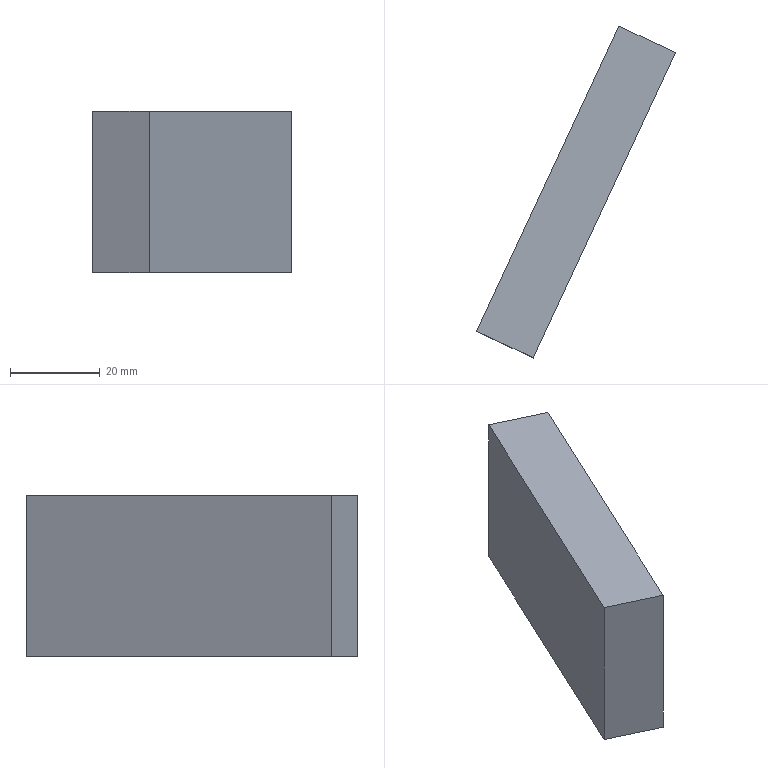Part | NX | features solid 2 | 1 solid | 6 faces | box 44.385 x 73.89 x 36 mm | volume 37800 mm3 | plane 6
STEP:
#1=CARTESIAN_POINT('',(-299.792,-21.721,9.));
#2=VERTEX_POINT('',#1);
#3=CARTESIAN_POINT('',(-312.48,-15.804,9.));
#4=VERTEX_POINT('',#3);
#5=CARTESIAN_POINT('',(-299.792,-21.721,9.));
#6=DIRECTION('',(-0.9063,0.4226,0.));
#7=VECTOR('',#6,1000.);
#8=LINE('',#5,#7);
#9=EDGE_CURVE('',#2,#4,#8,.T.);
#10=ORIENTED_EDGE('',*,*,#9,.T.);
#11=CARTESIAN_POINT('',(-312.48,-15.804,45.));
#12=VERTEX_POINT('',#11);
#13=CARTESIAN_POINT('',(-312.48,-15.804,45.));
#14=DIRECTION('',(0.,0.,-1.));
#15=VECTOR('',#14,1000.);
#16=LINE('',#13,#15);
#17=EDGE_CURVE('',#12,#4,#16,.T.);
#18=ORIENTED_EDGE('',*,*,#17,.F.);
#19=CARTESIAN_POINT('',(-299.792,-21.721,45.));
#20=VERTEX_POINT('',#19);
#21=CARTESIAN_POINT('',(-299.792,-21.721,45.));
#22=DIRECTION('',(-0.9063,0.4226,0.));
#23=VECTOR('',#22,1000.);
#24=LINE('',#21,#23);
#25=EDGE_CURVE('',#20,#12,#24,.T.);
#26=ORIENTED_EDGE('',*,*,#25,.F.);
#27=CARTESIAN_POINT('',(-299.792,-21.721,45.));
#28=DIRECTION('',(0.,0.,-1.));
#29=VECTOR('',#28,1000.);
#30=LINE('',#27,#29);
#31=EDGE_CURVE('',#20,#2,#30,.T.);
#32=ORIENTED_EDGE('',*,*,#31,.T.);
#33=EDGE_LOOP('',(#10,#18,#26,#32));
#34=FACE_BOUND('',#33,.T.);
#35=CARTESIAN_POINT('',(-299.792,-21.721,45.));
#36=DIRECTION('',(-0.4226,-0.9063,0.));
#37=DIRECTION('',(0.9063,-0.4226,0.));
#38=AXIS2_PLACEMENT_3D('',#35,#36,#37);
#39=PLANE('',#38);
#40=ADVANCED_FACE('',(#34),#39,.F.);
#41=CARTESIAN_POINT('',(-344.176,-83.777,9.));
#42=VERTEX_POINT('',#41);
#43=CARTESIAN_POINT('',(-312.48,-15.804,9.));
#44=DIRECTION('',(-0.4226,-0.9063,0.));
#45=VECTOR('',#44,1000.);
#46=LINE('',#43,#45);
#47=EDGE_CURVE('',#4,#42,#46,.T.);
#48=ORIENTED_EDGE('',*,*,#47,.T.);
#49=CARTESIAN_POINT('',(-344.176,-83.777,45.));
#50=VERTEX_POINT('',#49);
#51=CARTESIAN_POINT('',(-344.176,-83.777,45.));
#52=DIRECTION('',(0.,0.,-1.));
#53=VECTOR('',#52,1000.);
#54=LINE('',#51,#53);
#55=EDGE_CURVE('',#50,#42,#54,.T.);
#56=ORIENTED_EDGE('',*,*,#55,.F.);
#57=CARTESIAN_POINT('',(-312.48,-15.804,45.));
#58=DIRECTION('',(-0.4226,-0.9063,0.));
#59=VECTOR('',#58,1000.);
#60=LINE('',#57,#59);
#61=EDGE_CURVE('',#12,#50,#60,.T.);
#62=ORIENTED_EDGE('',*,*,#61,.F.);
#63=ORIENTED_EDGE('',*,*,#17,.T.);
#64=EDGE_LOOP('',(#48,#56,#62,#63));
#65=FACE_BOUND('',#64,.T.);
#66=CARTESIAN_POINT('',(-312.48,-15.804,45.));
#67=DIRECTION('',(0.9063,-0.4226,0.));
#68=DIRECTION('',(0.4226,0.9063,0.));
#69=AXIS2_PLACEMENT_3D('',#66,#67,#68);
#70=PLANE('',#69);
#71=ADVANCED_FACE('',(#65),#70,.F.);
#72=CARTESIAN_POINT('',(-331.488,-89.694,9.));
#73=VERTEX_POINT('',#72);
#74=CARTESIAN_POINT('',(-331.488,-89.694,9.));
#75=DIRECTION('',(-0.9063,0.4226,0.));
#76=VECTOR('',#75,1000.);
#77=LINE('',#74,#76);
#78=EDGE_CURVE('',#73,#42,#77,.T.);
#79=ORIENTED_EDGE('',*,*,#78,.F.);
#80=CARTESIAN_POINT('',(-331.488,-89.694,45.));
#81=VERTEX_POINT('',#80);
#82=CARTESIAN_POINT('',(-331.488,-89.694,45.));
#83=DIRECTION('',(0.,0.,-1.));
#84=VECTOR('',#83,1000.);
#85=LINE('',#82,#84);
#86=EDGE_CURVE('',#81,#73,#85,.T.);
#87=ORIENTED_EDGE('',*,*,#86,.F.);
#88=CARTESIAN_POINT('',(-331.488,-89.694,45.));
#89=DIRECTION('',(-0.9063,0.4226,0.));
#90=VECTOR('',#89,1000.);
#91=LINE('',#88,#90);
#92=EDGE_CURVE('',#81,#50,#91,.T.);
#93=ORIENTED_EDGE('',*,*,#92,.T.);
#94=ORIENTED_EDGE('',*,*,#55,.T.);
#95=EDGE_LOOP('',(#79,#87,#93,#94));
#96=FACE_BOUND('',#95,.T.);
#97=CARTESIAN_POINT('',(-331.488,-89.694,45.));
#98=DIRECTION('',(-0.4226,-0.9063,0.));
#99=DIRECTION('',(0.9063,-0.4226,0.));
#100=AXIS2_PLACEMENT_3D('',#97,#98,#99);
#101=PLANE('',#100);
#102=ADVANCED_FACE('',(#96),#101,.T.);
#103=CARTESIAN_POINT('',(-299.792,-21.721,9.));
#104=DIRECTION('',(-0.4226,-0.9063,0.));
#105=VECTOR('',#104,1000.);
#106=LINE('',#103,#105);
#107=EDGE_CURVE('',#2,#73,#106,.T.);
#108=ORIENTED_EDGE('',*,*,#107,.F.);
#109=ORIENTED_EDGE('',*,*,#31,.F.);
#110=CARTESIAN_POINT('',(-299.792,-21.721,45.));
#111=DIRECTION('',(-0.4226,-0.9063,0.));
#112=VECTOR('',#111,1000.);
#113=LINE('',#110,#112);
#114=EDGE_CURVE('',#20,#81,#113,.T.);
#115=ORIENTED_EDGE('',*,*,#114,.T.);
#116=ORIENTED_EDGE('',*,*,#86,.T.);
#117=EDGE_LOOP('',(#108,#109,#115,#116));
#118=FACE_BOUND('',#117,.T.);
#119=CARTESIAN_POINT('',(-299.792,-21.721,45.));
#120=DIRECTION('',(0.9063,-0.4226,0.));
#121=DIRECTION('',(0.4226,0.9063,0.));
#122=AXIS2_PLACEMENT_3D('',#119,#120,#121);
#123=PLANE('',#122);
#124=ADVANCED_FACE('',(#118),#123,.T.);
#125=ORIENTED_EDGE('',*,*,#25,.T.);
#126=ORIENTED_EDGE('',*,*,#61,.T.);
#127=ORIENTED_EDGE('',*,*,#92,.F.);
#128=ORIENTED_EDGE('',*,*,#114,.F.);
#129=EDGE_LOOP('',(#125,#126,#127,#128));
#130=FACE_BOUND('',#129,.T.);
#131=CARTESIAN_POINT('',(-312.48,-15.804,45.));
#132=DIRECTION('',(0.,0.,1.));
#133=DIRECTION('',(1.,0.,0.));
#134=AXIS2_PLACEMENT_3D('',#131,#132,#133);
#135=PLANE('',#134);
#136=ADVANCED_FACE('',(#130),#135,.T.);
#137=ORIENTED_EDGE('',*,*,#9,.F.);
#138=ORIENTED_EDGE('',*,*,#107,.T.);
#139=ORIENTED_EDGE('',*,*,#78,.T.);
#140=ORIENTED_EDGE('',*,*,#47,.F.);
#141=EDGE_LOOP('',(#137,#138,#139,#140));
#142=FACE_BOUND('',#141,.T.);
#143=CARTESIAN_POINT('',(-312.48,-15.804,9.));
#144=DIRECTION('',(0.,0.,1.));
#145=DIRECTION('',(1.,0.,0.));
#146=AXIS2_PLACEMENT_3D('',#143,#144,#145);
#147=PLANE('',#146);
#148=ADVANCED_FACE('',(#142),#147,.F.);
#149=CLOSED_SHELL('',(#40,#71,#102,#124,#136,#148));
#150=MANIFOLD_SOLID_BREP('',#149);
#151=(LENGTH_UNIT()NAMED_UNIT(*)SI_UNIT(.MILLI.,.METRE.));
#152=UNCERTAINTY_MEASURE_WITH_UNIT(LENGTH_MEASURE(0.00001),#151,'','');
#153=(NAMED_UNIT(*)PLANE_ANGLE_UNIT()SI_UNIT($,.RADIAN.));
#154=(NAMED_UNIT(*)SI_UNIT($,.STERADIAN.)SOLID_ANGLE_UNIT());
#155=(GEOMETRIC_REPRESENTATION_CONTEXT(3)GLOBAL_UNCERTAINTY_ASSIGNED_CONTEXT((#152))GLOBAL_UNIT_ASSIGNED_CONTEXT((#151,#153,#154))REPRESENTATION_CONTEXT('',''));
#156=ADVANCED_BREP_SHAPE_REPRESENTATION('',(#150),#155);